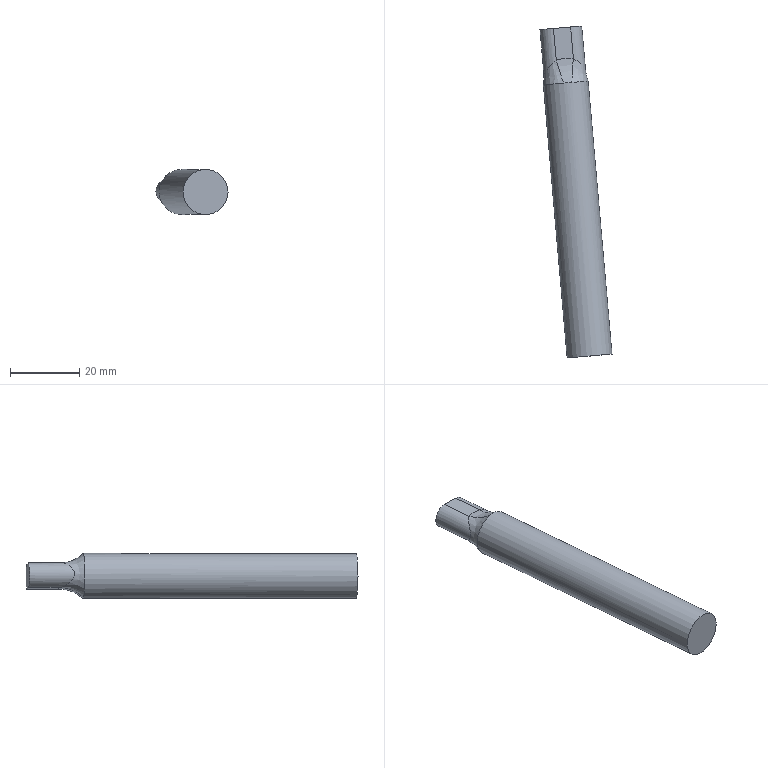Part | NX | features SPES 13-80-12.10-7.100 2 | 1 solid | 11 faces | box 20.77 x 95.731 x 13 mm | volume 11797 mm3 | plane 4 | spline 4 | cylinder 3 | commonest cylinder face diameters 7.1 x2 13 x1
STEP:
#1=CARTESIAN_POINT('',(713.61,-57.66,-43.192));
#2=VERTEX_POINT('',#1);
#3=CARTESIAN_POINT('',(712.816,-48.586,-43.192));
#4=VERTEX_POINT('',#3);
#5=CARTESIAN_POINT('',(714.207,-64.491,-43.192));
#6=DIRECTION('',(-0.08716,0.9962,0.));
#7=VECTOR('',#6,1000.);
#8=LINE('',#5,#7);
#9=EDGE_CURVE('',#2,#4,#8,.T.);
#10=ORIENTED_EDGE('',*,*,#9,.F.);
#11=CARTESIAN_POINT('',(714.299,-57.6,-36.125));
#12=VERTEX_POINT('',#11);
#13=CARTESIAN_POINT('',(713.61,-57.66,-43.192));
#14=CARTESIAN_POINT('',(713.178,-58.041,-43.146));
#15=CARTESIAN_POINT('',(712.379,-58.84,-42.879));
#16=CARTESIAN_POINT('',(711.454,-60.072,-42.077));
#17=CARTESIAN_POINT('',(710.952,-61.054,-41.133));
#18=CARTESIAN_POINT('',(710.751,-61.672,-40.173));
#19=CARTESIAN_POINT('',(710.744,-61.89,-39.304));
#20=CARTESIAN_POINT('',(710.92,-61.652,-38.459));
#21=CARTESIAN_POINT('',(711.3,-61.023,-37.575));
#22=CARTESIAN_POINT('',(711.975,-60.023,-36.759));
#23=CARTESIAN_POINT('',(713.035,-58.781,-36.174));
#24=CARTESIAN_POINT('',(713.867,-57.981,-36.08));
#25=CARTESIAN_POINT('',(714.299,-57.6,-36.125));
#26=B_SPLINE_CURVE_WITH_KNOTS('',3,(#13,#14,#15,#16,#17,#18,#19,#20,#21,#22,#23,#24,#25),.UNSPECIFIED.,.F.,.F.,(4,1,1,1,1,1,1,1,1,1,4),(0.,0.001722,0.003444,0.005167,0.006028,0.006889,0.00775,0.008611,0.01033,0.01206,0.01378),.UNSPECIFIED.);
#27=EDGE_CURVE('',#2,#12,#26,.T.);
#28=ORIENTED_EDGE('',*,*,#27,.T.);
#29=CARTESIAN_POINT('',(713.505,-48.525,-36.125));
#30=VERTEX_POINT('',#29);
#31=CARTESIAN_POINT('',(714.896,-64.431,-36.125));
#32=DIRECTION('',(-0.08716,0.9962,0.));
#33=VECTOR('',#32,1000.);
#34=LINE('',#31,#33);
#35=EDGE_CURVE('',#12,#30,#34,.T.);
#36=ORIENTED_EDGE('',*,*,#35,.T.);
#37=CARTESIAN_POINT('',(713.16,-48.555,-39.659));
#38=DIRECTION('',(0.08716,-0.9962,0.));
#39=DIRECTION('',(0.9962,0.08716,0.));
#40=AXIS2_PLACEMENT_3D('',#37,#38,#39);
#41=CIRCLE('',#40,3.55);
#42=EDGE_CURVE('',#30,#4,#41,.T.);
#43=ORIENTED_EDGE('',*,*,#42,.T.);
#44=EDGE_LOOP('',(#10,#28,#36,#43));
#45=FACE_BOUND('',#44,.T.);
#46=CARTESIAN_POINT('',(714.552,-64.461,-39.659));
#47=DIRECTION('',(-0.08716,0.9962,0.));
#48=DIRECTION('',(-0.9962,-0.08716,0.));
#49=AXIS2_PLACEMENT_3D('',#46,#47,#48);
#50=CYLINDRICAL_SURFACE('',#49,3.55);
#51=ADVANCED_FACE('',(#45),#50,.T.);
#52=CARTESIAN_POINT('',(718.567,-57.226,-43.679));
#53=VERTEX_POINT('',#52);
#54=CARTESIAN_POINT('',(717.773,-48.152,-43.679));
#55=VERTEX_POINT('',#54);
#56=CARTESIAN_POINT('',(719.165,-64.057,-43.679));
#57=DIRECTION('',(-0.08716,0.9962,0.));
#58=VECTOR('',#57,1000.);
#59=LINE('',#56,#58);
#60=EDGE_CURVE('',#53,#55,#59,.T.);
#61=ORIENTED_EDGE('',*,*,#60,.F.);
#62=CARTESIAN_POINT('',(718.567,-57.226,-43.679));
#63=CARTESIAN_POINT('',(716.9,-57.052,-43.518));
#64=CARTESIAN_POINT('',(715.222,-57.199,-43.353));
#65=CARTESIAN_POINT('',(713.61,-57.66,-43.192));
#66=B_SPLINE_CURVE_WITH_KNOTS('',3,(#62,#63,#64,#65),.UNSPECIFIED.,.F.,.F.,(4,4),(0.,0.005042),.UNSPECIFIED.);
#67=EDGE_CURVE('',#53,#2,#66,.T.);
#68=ORIENTED_EDGE('',*,*,#67,.T.);
#69=ORIENTED_EDGE('',*,*,#9,.T.);
#70=CARTESIAN_POINT('',(717.773,-48.152,-43.679));
#71=DIRECTION('',(-0.9915,-0.08674,0.09739));
#72=VECTOR('',#71,1000.);
#73=LINE('',#70,#72);
#74=EDGE_CURVE('',#55,#4,#73,.T.);
#75=ORIENTED_EDGE('',*,*,#74,.F.);
#76=EDGE_LOOP('',(#61,#68,#69,#75));
#77=FACE_BOUND('',#76,.T.);
#78=CARTESIAN_POINT('',(719.165,-64.057,-43.679));
#79=DIRECTION('',(-0.09702,-0.008488,-0.9952));
#80=DIRECTION('',(-0.9953,0.,0.09702));
#81=AXIS2_PLACEMENT_3D('',#78,#79,#80);
#82=PLANE('',#81);
#83=ADVANCED_FACE('',(#77),#82,.T.);
#84=CARTESIAN_POINT('',(719.256,-57.166,-36.612));
#85=VERTEX_POINT('',#84);
#86=CARTESIAN_POINT('',(718.462,-48.092,-36.612));
#87=VERTEX_POINT('',#86);
#88=CARTESIAN_POINT('',(719.854,-63.997,-36.612));
#89=DIRECTION('',(-0.08716,0.9962,0.));
#90=VECTOR('',#89,1000.);
#91=LINE('',#88,#90);
#92=EDGE_CURVE('',#85,#87,#91,.T.);
#93=ORIENTED_EDGE('',*,*,#92,.F.);
#94=CARTESIAN_POINT('',(719.256,-57.166,-36.612));
#95=CARTESIAN_POINT('',(719.747,-57.466,-36.658));
#96=CARTESIAN_POINT('',(720.673,-58.115,-36.925));
#97=CARTESIAN_POINT('',(721.798,-59.167,-37.727));
#98=CARTESIAN_POINT('',(722.462,-60.047,-38.671));
#99=CARTESIAN_POINT('',(722.768,-60.62,-39.631));
#100=CARTESIAN_POINT('',(722.813,-60.834,-40.5));
#101=CARTESIAN_POINT('',(722.598,-60.631,-41.345));
#102=CARTESIAN_POINT('',(722.115,-60.076,-42.229));
#103=CARTESIAN_POINT('',(721.276,-59.209,-43.045));
#104=CARTESIAN_POINT('',(720.017,-58.17,-43.63));
#105=CARTESIAN_POINT('',(719.058,-57.526,-43.724));
#106=CARTESIAN_POINT('',(718.567,-57.226,-43.679));
#107=B_SPLINE_CURVE_WITH_KNOTS('',3,(#94,#95,#96,#97,#98,#99,#100,#101,#102,#103,#104,#105,#106),.UNSPECIFIED.,.F.,.F.,(4,1,1,1,1,1,1,1,1,1,4),(0.,0.001722,0.003444,0.005167,0.006028,0.006889,0.00775,0.008611,0.01033,0.01206,0.01378),.UNSPECIFIED.);
#108=EDGE_CURVE('',#85,#53,#107,.T.);
#109=ORIENTED_EDGE('',*,*,#108,.T.);
#110=ORIENTED_EDGE('',*,*,#60,.T.);
#111=CARTESIAN_POINT('',(718.118,-48.122,-40.146));
#112=DIRECTION('',(0.08716,-0.9962,0.));
#113=DIRECTION('',(0.9962,0.08716,0.));
#114=AXIS2_PLACEMENT_3D('',#111,#112,#113);
#115=CIRCLE('',#114,3.55);
#116=EDGE_CURVE('',#55,#87,#115,.T.);
#117=ORIENTED_EDGE('',*,*,#116,.T.);
#118=EDGE_LOOP('',(#93,#109,#110,#117));
#119=FACE_BOUND('',#118,.T.);
#120=CARTESIAN_POINT('',(719.509,-64.027,-40.146));
#121=DIRECTION('',(-0.08716,0.9962,0.));
#122=DIRECTION('',(-0.9962,-0.08716,0.));
#123=AXIS2_PLACEMENT_3D('',#120,#121,#122);
#124=CYLINDRICAL_SURFACE('',#123,3.55);
#125=ADVANCED_FACE('',(#119),#124,.T.);
#126=ORIENTED_EDGE('',*,*,#35,.F.);
#127=CARTESIAN_POINT('',(714.299,-57.6,-36.125));
#128=CARTESIAN_POINT('',(715.91,-57.139,-36.286));
#129=CARTESIAN_POINT('',(717.588,-56.992,-36.451));
#130=CARTESIAN_POINT('',(719.256,-57.166,-36.612));
#131=B_SPLINE_CURVE_WITH_KNOTS('',3,(#127,#128,#129,#130),.UNSPECIFIED.,.F.,.F.,(4,4),(0.,0.005042),.UNSPECIFIED.);
#132=EDGE_CURVE('',#12,#85,#131,.T.);
#133=ORIENTED_EDGE('',*,*,#132,.T.);
#134=ORIENTED_EDGE('',*,*,#92,.T.);
#135=CARTESIAN_POINT('',(718.462,-48.092,-36.612));
#136=DIRECTION('',(-0.9915,-0.08674,0.09739));
#137=VECTOR('',#136,1000.);
#138=LINE('',#135,#137);
#139=EDGE_CURVE('',#87,#30,#138,.T.);
#140=ORIENTED_EDGE('',*,*,#139,.T.);
#141=EDGE_LOOP('',(#126,#133,#134,#140));
#142=FACE_BOUND('',#141,.T.);
#143=CARTESIAN_POINT('',(719.854,-63.997,-36.612));
#144=DIRECTION('',(-0.09702,-0.008488,-0.9952));
#145=DIRECTION('',(-0.9953,0.,0.09702));
#146=AXIS2_PLACEMENT_3D('',#143,#144,#145);
#147=PLANE('',#146);
#148=ADVANCED_FACE('',(#142),#147,.F.);
#149=ORIENTED_EDGE('',*,*,#42,.F.);
#150=ORIENTED_EDGE('',*,*,#139,.F.);
#151=ORIENTED_EDGE('',*,*,#116,.F.);
#152=ORIENTED_EDGE('',*,*,#74,.T.);
#153=EDGE_LOOP('',(#149,#150,#151,#152));
#154=FACE_BOUND('',#153,.T.);
#155=CARTESIAN_POINT('',(713.16,-48.555,-39.659));
#156=DIRECTION('',(0.08716,-0.9962,0.));
#157=DIRECTION('',(0.9962,0.08716,0.));
#158=AXIS2_PLACEMENT_3D('',#155,#156,#157);
#159=PLANE('',#158);
#160=ADVANCED_FACE('',(#154),#159,.F.);
#161=CARTESIAN_POINT('',(730.394,-142.411,-39.902));
#162=VERTEX_POINT('',#161);
#163=CARTESIAN_POINT('',(723.919,-142.977,-39.902));
#164=DIRECTION('',(0.08716,-0.9962,0.));
#165=DIRECTION('',(0.9962,0.08716,0.));
#166=AXIS2_PLACEMENT_3D('',#163,#164,#165);
#167=CIRCLE('',#166,6.5);
#168=EDGE_CURVE('',#162,#162,#167,.F.);
#169=ORIENTED_EDGE('',*,*,#168,.F.);
#170=EDGE_LOOP('',(#169));
#171=FACE_BOUND('',#170,.T.);
#172=CARTESIAN_POINT('',(723.919,-142.977,-39.902));
#173=DIRECTION('',(0.08716,-0.9962,0.));
#174=DIRECTION('',(0.9962,0.08716,0.));
#175=AXIS2_PLACEMENT_3D('',#172,#173,#174);
#176=PLANE('',#175);
#177=ADVANCED_FACE('',(#171),#176,.T.);
#178=ORIENTED_EDGE('',*,*,#168,.T.);
#179=EDGE_LOOP('',(#178));
#180=FACE_BOUND('',#179,.T.);
#181=CARTESIAN_POINT('',(718.82,-64.087,-33.655));
#182=VERTEX_POINT('',#181);
#183=CARTESIAN_POINT('',(716.481,-64.292,-33.425));
#184=VERTEX_POINT('',#183);
#185=CARTESIAN_POINT('',(717.031,-64.244,-39.902));
#186=DIRECTION('',(0.08716,-0.9962,0.));
#187=DIRECTION('',(0.9962,0.08716,0.));
#188=AXIS2_PLACEMENT_3D('',#185,#186,#187);
#189=CIRCLE('',#188,6.5);
#190=EDGE_CURVE('',#182,#184,#189,.T.);
#191=ORIENTED_EDGE('',*,*,#190,.T.);
#192=CARTESIAN_POINT('',(715.241,-64.4,-46.149));
#193=VERTEX_POINT('',#192);
#194=CARTESIAN_POINT('',(717.031,-64.244,-39.902));
#195=DIRECTION('',(0.08716,-0.9962,0.));
#196=DIRECTION('',(0.9962,0.08716,0.));
#197=AXIS2_PLACEMENT_3D('',#194,#195,#196);
#198=CIRCLE('',#197,6.5);
#199=EDGE_CURVE('',#184,#193,#198,.T.);
#200=ORIENTED_EDGE('',*,*,#199,.T.);
#201=CARTESIAN_POINT('',(717.58,-64.196,-46.379));
#202=VERTEX_POINT('',#201);
#203=CARTESIAN_POINT('',(717.031,-64.244,-39.902));
#204=DIRECTION('',(0.08716,-0.9962,0.));
#205=DIRECTION('',(0.9962,0.08716,0.));
#206=AXIS2_PLACEMENT_3D('',#203,#204,#205);
#207=CIRCLE('',#206,6.5);
#208=EDGE_CURVE('',#193,#202,#207,.T.);
#209=ORIENTED_EDGE('',*,*,#208,.T.);
#210=CARTESIAN_POINT('',(717.031,-64.244,-39.902));
#211=DIRECTION('',(0.08716,-0.9962,0.));
#212=DIRECTION('',(0.9962,0.08716,0.));
#213=AXIS2_PLACEMENT_3D('',#210,#211,#212);
#214=CIRCLE('',#213,6.5);
#215=EDGE_CURVE('',#202,#182,#214,.T.);
#216=ORIENTED_EDGE('',*,*,#215,.T.);
#217=EDGE_LOOP('',(#191,#200,#209,#216));
#218=FACE_BOUND('',#217,.T.);
#219=CARTESIAN_POINT('',(717.031,-64.244,-39.902));
#220=DIRECTION('',(0.08716,-0.9962,0.));
#221=DIRECTION('',(0.9962,0.08716,0.));
#222=AXIS2_PLACEMENT_3D('',#219,#220,#221);
#223=CYLINDRICAL_SURFACE('',#222,6.5);
#224=ADVANCED_FACE('',(#180,#218),#223,.T.);
#225=CARTESIAN_POINT('',(715.269,-57.515,-26.173));
#226=DIRECTION('',(0.9571,0.2736,-0.09563));
#227=DIRECTION('',(-0.2748,0.9615,0.));
#228=AXIS2_PLACEMENT_3D('',#225,#226,#227);
#229=CIRCLE('',#228,10.);
#230=EDGE_CURVE('',#184,#12,#229,.T.);
#231=ORIENTED_EDGE('',*,*,#230,.F.);
#232=ORIENTED_EDGE('',*,*,#190,.F.);
#233=CARTESIAN_POINT('',(720.226,-57.081,-26.66));
#234=DIRECTION('',(0.9901,-0.1032,-0.09563));
#235=DIRECTION('',(0.1037,0.9946,0.));
#236=AXIS2_PLACEMENT_3D('',#233,#234,#235);
#237=CIRCLE('',#236,10.);
#238=EDGE_CURVE('',#85,#182,#237,.F.);
#239=ORIENTED_EDGE('',*,*,#238,.F.);
#240=ORIENTED_EDGE('',*,*,#132,.F.);
#241=EDGE_LOOP('',(#231,#232,#239,#240));
#242=FACE_BOUND('',#241,.T.);
#243=CARTESIAN_POINT('',(718.82,-64.087,-33.655));
#244=CARTESIAN_POINT('',(718.841,-61.214,-36.537));
#245=CARTESIAN_POINT('',(719.256,-57.166,-36.612));
#246=CARTESIAN_POINT('',(718.088,-64.151,-33.444));
#247=CARTESIAN_POINT('',(717.706,-61.212,-36.427));
#248=CARTESIAN_POINT('',(717.594,-56.993,-36.452));
#249=CARTESIAN_POINT('',(717.236,-64.226,-33.361));
#250=CARTESIAN_POINT('',(716.522,-61.317,-36.31));
#251=CARTESIAN_POINT('',(715.895,-57.143,-36.285));
#252=CARTESIAN_POINT('',(716.481,-64.292,-33.425));
#253=CARTESIAN_POINT('',(715.41,-61.514,-36.2));
#254=CARTESIAN_POINT('',(714.299,-57.6,-36.125));
#255=(BOUNDED_SURFACE()B_SPLINE_SURFACE(3,2,((#243,#244,#245),(#246,#247,#248),(#249,#250,#251),(#252,#253,#254)),.UNSPECIFIED.,.F.,.F.,.F.)B_SPLINE_SURFACE_WITH_KNOTS((4,4),(3,3),(0.01051,0.01554),(0.,1.),.PIECEWISE_BEZIER_KNOTS.)GEOMETRIC_REPRESENTATION_ITEM()RATIONAL_B_SPLINE_SURFACE(((1.,0.9262,1.),(1.,0.9225,1.),(1.,0.9225,1.),(1.,0.9262,1.)))REPRESENTATION_ITEM('')SURFACE());
#256=ADVANCED_FACE('',(#242),#255,.F.);
#257=ORIENTED_EDGE('',*,*,#238,.T.);
#258=ORIENTED_EDGE('',*,*,#215,.F.);
#259=CARTESIAN_POINT('',(717.597,-57.311,-53.631));
#260=DIRECTION('',(-0.9901,0.1032,0.09563));
#261=DIRECTION('',(-0.1037,-0.9946,0.));
#262=AXIS2_PLACEMENT_3D('',#259,#260,#261);
#263=CIRCLE('',#262,10.);
#264=EDGE_CURVE('',#53,#202,#263,.F.);
#265=ORIENTED_EDGE('',*,*,#264,.F.);
#266=ORIENTED_EDGE('',*,*,#108,.F.);
#267=EDGE_LOOP('',(#257,#258,#265,#266));
#268=FACE_BOUND('',#267,.T.);
#269=CARTESIAN_POINT('',(717.58,-64.196,-46.379));
#270=CARTESIAN_POINT('',(718.152,-61.274,-43.604));
#271=CARTESIAN_POINT('',(718.567,-57.226,-43.679));
#272=CARTESIAN_POINT('',(719.22,-64.052,-46.239));
#273=CARTESIAN_POINT('',(719.05,-61.329,-43.89));
#274=CARTESIAN_POINT('',(719.552,-57.829,-43.77));
#275=CARTESIAN_POINT('',(721.355,-63.866,-45.119));
#276=CARTESIAN_POINT('',(720.746,-61.594,-43.763));
#277=CARTESIAN_POINT('',(721.071,-58.959,-43.332));
#278=CARTESIAN_POINT('',(723.011,-63.721,-42.698));
#279=CARTESIAN_POINT('',(722.438,-62.13,-42.184));
#280=CARTESIAN_POINT('',(722.405,-60.4,-41.886));
#281=CARTESIAN_POINT('',(723.6,-63.669,-40.545));
#282=CARTESIAN_POINT('',(723.05,-62.355,-40.503));
#283=CARTESIAN_POINT('',(722.884,-60.953,-40.499));
#284=CARTESIAN_POINT('',(723.438,-63.683,-38.327));
#285=CARTESIAN_POINT('',(722.775,-62.101,-38.747));
#286=CARTESIAN_POINT('',(722.681,-60.377,-39.061));
#287=CARTESIAN_POINT('',(722.28,-63.785,-35.621));
#288=CARTESIAN_POINT('',(721.416,-61.535,-36.873));
#289=CARTESIAN_POINT('',(721.647,-58.907,-37.404));
#290=CARTESIAN_POINT('',(720.395,-63.95,-34.11));
#291=CARTESIAN_POINT('',(719.773,-61.265,-36.429));
#292=CARTESIAN_POINT('',(720.236,-57.766,-36.703));
#293=CARTESIAN_POINT('',(718.82,-64.087,-33.655));
#294=CARTESIAN_POINT('',(718.841,-61.214,-36.537));
#295=CARTESIAN_POINT('',(719.256,-57.166,-36.612));
#296=(BOUNDED_SURFACE()B_SPLINE_SURFACE(3,2,((#269,#270,#271),(#272,#273,#274),(#275,#276,#277),(#278,#279,#280),(#281,#282,#283),(#284,#285,#286),(#287,#288,#289),(#290,#291,#292),(#293,#294,#295)),.UNSPECIFIED.,.F.,.F.,.F.)B_SPLINE_SURFACE_WITH_KNOTS((4,1,1,1,1,1,4),(3,3),(0.02315,0.03394,0.03933,0.04472,0.05012,0.05551,0.06629),(0.,1.),.UNSPECIFIED.)GEOMETRIC_REPRESENTATION_ITEM()RATIONAL_B_SPLINE_SURFACE(((1.,0.9262,1.),(1.,0.9437,1.),(1.,0.9676,1.),(1.,0.9854,1.),(1.,0.9903,1.),(1.,0.9855,1.),(1.,0.9676,1.),(1.,0.9436,1.),(1.,0.9262,1.)))REPRESENTATION_ITEM('')SURFACE());
#297=ADVANCED_FACE('',(#268),#296,.F.);
#298=ORIENTED_EDGE('',*,*,#230,.T.);
#299=ORIENTED_EDGE('',*,*,#27,.F.);
#300=CARTESIAN_POINT('',(712.64,-57.745,-53.144));
#301=DIRECTION('',(-0.9571,-0.2736,0.09563));
#302=DIRECTION('',(0.2748,-0.9615,0.));
#303=AXIS2_PLACEMENT_3D('',#300,#301,#302);
#304=CIRCLE('',#303,10.);
#305=EDGE_CURVE('',#193,#2,#304,.T.);
#306=ORIENTED_EDGE('',*,*,#305,.F.);
#307=ORIENTED_EDGE('',*,*,#199,.F.);
#308=EDGE_LOOP('',(#298,#299,#306,#307));
#309=FACE_BOUND('',#308,.T.);
#310=CARTESIAN_POINT('',(716.481,-64.292,-33.425));
#311=CARTESIAN_POINT('',(715.41,-61.514,-36.2));
#312=CARTESIAN_POINT('',(714.299,-57.6,-36.125));
#313=CARTESIAN_POINT('',(714.841,-64.435,-33.566));
#314=CARTESIAN_POINT('',(714.536,-61.724,-35.914));
#315=CARTESIAN_POINT('',(713.433,-58.364,-36.035));
#316=CARTESIAN_POINT('',(712.706,-64.622,-34.685));
#317=CARTESIAN_POINT('',(712.911,-62.28,-36.041));
#318=CARTESIAN_POINT('',(712.134,-59.741,-36.472));
#319=CARTESIAN_POINT('',(711.05,-64.767,-37.106));
#320=CARTESIAN_POINT('',(711.338,-63.101,-37.62));
#321=CARTESIAN_POINT('',(711.07,-61.391,-37.918));
#322=CARTESIAN_POINT('',(710.461,-64.819,-39.259));
#323=CARTESIAN_POINT('',(710.775,-63.429,-39.301));
#324=CARTESIAN_POINT('',(710.694,-62.019,-39.305));
#325=CARTESIAN_POINT('',(710.623,-64.805,-41.477));
#326=CARTESIAN_POINT('',(711.002,-63.131,-41.058));
#327=CARTESIAN_POINT('',(710.794,-61.416,-40.743));
#328=CARTESIAN_POINT('',(711.781,-64.703,-44.183));
#329=CARTESIAN_POINT('',(712.241,-62.337,-42.931));
#330=CARTESIAN_POINT('',(711.557,-59.789,-42.4));
#331=CARTESIAN_POINT('',(713.666,-64.538,-45.694));
#332=CARTESIAN_POINT('',(713.813,-61.787,-43.375));
#333=CARTESIAN_POINT('',(712.748,-58.421,-43.101));
#334=CARTESIAN_POINT('',(715.241,-64.4,-46.149));
#335=CARTESIAN_POINT('',(714.721,-61.574,-43.267));
#336=CARTESIAN_POINT('',(713.61,-57.66,-43.192));
#337=(BOUNDED_SURFACE()B_SPLINE_SURFACE(3,2,((#310,#311,#312),(#313,#314,#315),(#316,#317,#318),(#319,#320,#321),(#322,#323,#324),(#325,#326,#327),(#328,#329,#330),(#331,#332,#333),(#334,#335,#336)),.UNSPECIFIED.,.F.,.F.,.F.)B_SPLINE_SURFACE_WITH_KNOTS((4,1,1,1,1,1,4),(3,3),(0.02315,0.03394,0.03933,0.04472,0.05012,0.05551,0.06629),(0.,1.),.UNSPECIFIED.)GEOMETRIC_REPRESENTATION_ITEM()RATIONAL_B_SPLINE_SURFACE(((1.,0.9262,1.),(1.,0.9437,1.),(1.,0.9676,1.),(1.,0.9854,1.),(1.,0.9903,1.),(1.,0.9855,1.),(1.,0.9676,1.),(1.,0.9436,1.),(1.,0.9262,1.)))REPRESENTATION_ITEM('')SURFACE());
#338=ADVANCED_FACE('',(#309),#337,.F.);
#339=ORIENTED_EDGE('',*,*,#264,.T.);
#340=ORIENTED_EDGE('',*,*,#208,.F.);
#341=ORIENTED_EDGE('',*,*,#305,.T.);
#342=ORIENTED_EDGE('',*,*,#67,.F.);
#343=EDGE_LOOP('',(#339,#340,#341,#342));
#344=FACE_BOUND('',#343,.T.);
#345=CARTESIAN_POINT('',(715.241,-64.4,-46.149));
#346=CARTESIAN_POINT('',(714.721,-61.574,-43.267));
#347=CARTESIAN_POINT('',(713.61,-57.66,-43.192));
#348=CARTESIAN_POINT('',(715.973,-64.336,-46.36));
#349=CARTESIAN_POINT('',(715.839,-61.376,-43.377));
#350=CARTESIAN_POINT('',(715.216,-57.201,-43.352));
#351=CARTESIAN_POINT('',(716.825,-64.262,-46.443));
#352=CARTESIAN_POINT('',(717.023,-61.273,-43.494));
#353=CARTESIAN_POINT('',(716.915,-57.054,-43.519));
#354=CARTESIAN_POINT('',(717.58,-64.196,-46.379));
#355=CARTESIAN_POINT('',(718.152,-61.274,-43.604));
#356=CARTESIAN_POINT('',(718.567,-57.226,-43.679));
#357=(BOUNDED_SURFACE()B_SPLINE_SURFACE(3,2,((#345,#346,#347),(#348,#349,#350),(#351,#352,#353),(#354,#355,#356)),.UNSPECIFIED.,.F.,.F.,.F.)B_SPLINE_SURFACE_WITH_KNOTS((4,4),(3,3),(0.01051,0.01554),(0.,1.),.PIECEWISE_BEZIER_KNOTS.)GEOMETRIC_REPRESENTATION_ITEM()RATIONAL_B_SPLINE_SURFACE(((1.,0.9262,1.),(1.,0.9225,1.),(1.,0.9225,1.),(1.,0.9262,1.)))REPRESENTATION_ITEM('')SURFACE());
#358=ADVANCED_FACE('',(#344),#357,.F.);
#359=CLOSED_SHELL('',(#51,#83,#125,#148,#160,#177,#224,#256,#297,#338,#358));
#360=MANIFOLD_SOLID_BREP('',#359);
#361=(LENGTH_UNIT()NAMED_UNIT(*)SI_UNIT(.MILLI.,.METRE.));
#362=UNCERTAINTY_MEASURE_WITH_UNIT(LENGTH_MEASURE(0.0508),#361,'','');
#363=(NAMED_UNIT(*)PLANE_ANGLE_UNIT()SI_UNIT($,.RADIAN.));
#364=(NAMED_UNIT(*)SI_UNIT($,.STERADIAN.)SOLID_ANGLE_UNIT());
#365=(GEOMETRIC_REPRESENTATION_CONTEXT(3)GLOBAL_UNCERTAINTY_ASSIGNED_CONTEXT((#362))GLOBAL_UNIT_ASSIGNED_CONTEXT((#361,#363,#364))REPRESENTATION_CONTEXT('',''));
#366=ADVANCED_BREP_SHAPE_REPRESENTATION('',(#360),#365);